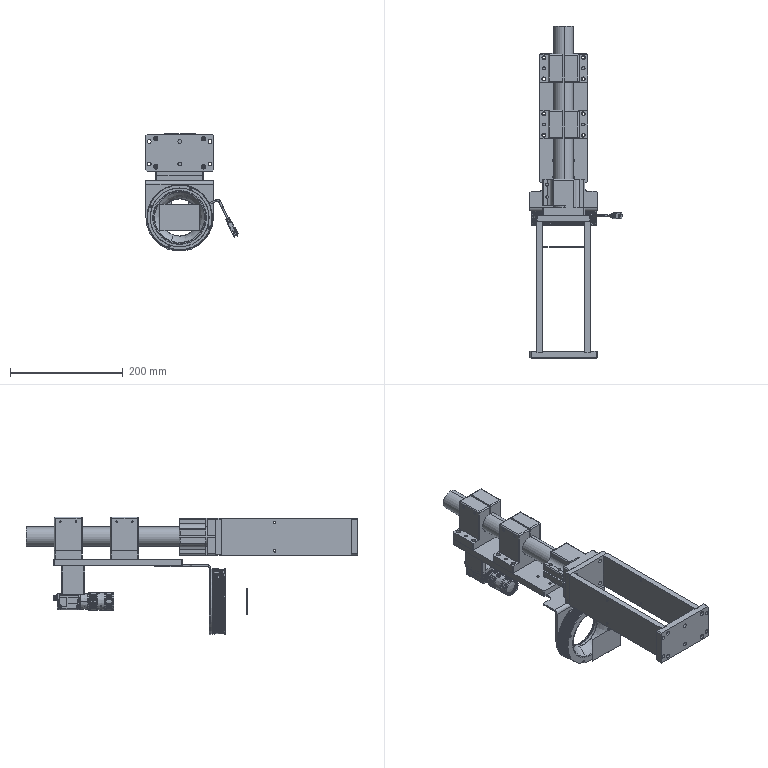Part | SolidWorks | features 3DProfileFeature 1 | 18 solids | 4503 faces | volume 1570988 mm3 | plane 1923 | cylinder 1332 | spline 826 | cone 399 | torus 13 | sphere 10 | commonest cylinder face diameters 0.6 x141 4 x114 0.4 x86 1 x57 0.7 x45 4.5 x44